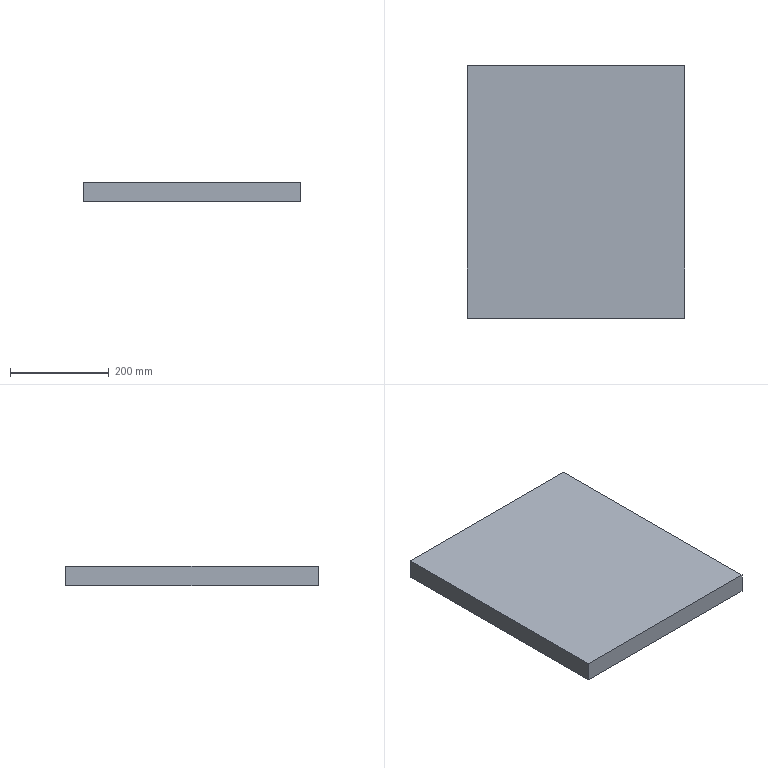Part | SolidWorks | features Extrusion 1 | 1 solid | 6 faces | box 440 x 510 x 40 mm | volume 8976000 mm3 | plane 6
STEP:
#1=CARTESIAN_POINT('',(0.,510.,0.));
#2=VERTEX_POINT('',#1);
#3=CARTESIAN_POINT('',(0.,0.,0.));
#4=VERTEX_POINT('',#3);
#5=CARTESIAN_POINT('',(0.,0.,0.));
#6=DIRECTION('',(0.,-1.,0.));
#7=VECTOR('',#6,1000.);
#8=LINE('',#5,#7);
#9=EDGE_CURVE('',#2,#4,#8,.T.);
#10=ORIENTED_EDGE('',*,*,#9,.T.);
#11=CARTESIAN_POINT('',(0.,0.,40.));
#12=VERTEX_POINT('',#11);
#13=CARTESIAN_POINT('',(0.,0.,40.));
#14=DIRECTION('',(0.,0.,-1.));
#15=VECTOR('',#14,1000.);
#16=LINE('',#13,#15);
#17=EDGE_CURVE('',#12,#4,#16,.T.);
#18=ORIENTED_EDGE('',*,*,#17,.F.);
#19=CARTESIAN_POINT('',(0.,510.,40.));
#20=VERTEX_POINT('',#19);
#21=CARTESIAN_POINT('',(0.,0.,40.));
#22=DIRECTION('',(0.,-1.,0.));
#23=VECTOR('',#22,1000.);
#24=LINE('',#21,#23);
#25=EDGE_CURVE('',#20,#12,#24,.T.);
#26=ORIENTED_EDGE('',*,*,#25,.F.);
#27=CARTESIAN_POINT('',(0.,510.,40.));
#28=DIRECTION('',(0.,0.,-1.));
#29=VECTOR('',#28,1000.);
#30=LINE('',#27,#29);
#31=EDGE_CURVE('',#20,#2,#30,.T.);
#32=ORIENTED_EDGE('',*,*,#31,.T.);
#33=EDGE_LOOP('',(#10,#18,#26,#32));
#34=FACE_OUTER_BOUND('',#33,.T.);
#35=CARTESIAN_POINT('',(0.,0.,40.));
#36=DIRECTION('',(1.,0.,0.));
#37=DIRECTION('',(0.,0.,-1.));
#38=AXIS2_PLACEMENT_3D('',#35,#36,#37);
#39=PLANE('',#38);
#40=ADVANCED_FACE('',(#34),#39,.F.);
#41=CARTESIAN_POINT('',(440.,0.,0.));
#42=VERTEX_POINT('',#41);
#43=CARTESIAN_POINT('',(0.,0.,0.));
#44=DIRECTION('',(1.,0.,0.));
#45=VECTOR('',#44,1000.);
#46=LINE('',#43,#45);
#47=EDGE_CURVE('',#4,#42,#46,.T.);
#48=ORIENTED_EDGE('',*,*,#47,.T.);
#49=CARTESIAN_POINT('',(440.,0.,40.));
#50=VERTEX_POINT('',#49);
#51=CARTESIAN_POINT('',(440.,0.,40.));
#52=DIRECTION('',(0.,0.,-1.));
#53=VECTOR('',#52,1000.);
#54=LINE('',#51,#53);
#55=EDGE_CURVE('',#50,#42,#54,.T.);
#56=ORIENTED_EDGE('',*,*,#55,.F.);
#57=CARTESIAN_POINT('',(0.,0.,40.));
#58=DIRECTION('',(1.,0.,0.));
#59=VECTOR('',#58,1000.);
#60=LINE('',#57,#59);
#61=EDGE_CURVE('',#12,#50,#60,.T.);
#62=ORIENTED_EDGE('',*,*,#61,.F.);
#63=ORIENTED_EDGE('',*,*,#17,.T.);
#64=EDGE_LOOP('',(#48,#56,#62,#63));
#65=FACE_OUTER_BOUND('',#64,.T.);
#66=CARTESIAN_POINT('',(0.,0.,40.));
#67=DIRECTION('',(0.,1.,0.));
#68=DIRECTION('',(0.,0.,1.));
#69=AXIS2_PLACEMENT_3D('',#66,#67,#68);
#70=PLANE('',#69);
#71=ADVANCED_FACE('',(#65),#70,.F.);
#72=CARTESIAN_POINT('',(440.,510.,0.));
#73=VERTEX_POINT('',#72);
#74=CARTESIAN_POINT('',(440.,0.,0.));
#75=DIRECTION('',(0.,1.,0.));
#76=VECTOR('',#75,1000.);
#77=LINE('',#74,#76);
#78=EDGE_CURVE('',#42,#73,#77,.T.);
#79=ORIENTED_EDGE('',*,*,#78,.T.);
#80=CARTESIAN_POINT('',(440.,510.,40.));
#81=VERTEX_POINT('',#80);
#82=CARTESIAN_POINT('',(440.,510.,40.));
#83=DIRECTION('',(0.,0.,-1.));
#84=VECTOR('',#83,1000.);
#85=LINE('',#82,#84);
#86=EDGE_CURVE('',#81,#73,#85,.T.);
#87=ORIENTED_EDGE('',*,*,#86,.F.);
#88=CARTESIAN_POINT('',(440.,0.,40.));
#89=DIRECTION('',(0.,1.,0.));
#90=VECTOR('',#89,1000.);
#91=LINE('',#88,#90);
#92=EDGE_CURVE('',#50,#81,#91,.T.);
#93=ORIENTED_EDGE('',*,*,#92,.F.);
#94=ORIENTED_EDGE('',*,*,#55,.T.);
#95=EDGE_LOOP('',(#79,#87,#93,#94));
#96=FACE_OUTER_BOUND('',#95,.T.);
#97=CARTESIAN_POINT('',(440.,0.,40.));
#98=DIRECTION('',(-1.,0.,0.));
#99=DIRECTION('',(0.,0.,1.));
#100=AXIS2_PLACEMENT_3D('',#97,#98,#99);
#101=PLANE('',#100);
#102=ADVANCED_FACE('',(#96),#101,.F.);
#103=CARTESIAN_POINT('',(0.,510.,0.));
#104=DIRECTION('',(-1.,0.,0.));
#105=VECTOR('',#104,1000.);
#106=LINE('',#103,#105);
#107=EDGE_CURVE('',#73,#2,#106,.T.);
#108=ORIENTED_EDGE('',*,*,#107,.T.);
#109=ORIENTED_EDGE('',*,*,#31,.F.);
#110=CARTESIAN_POINT('',(0.,510.,40.));
#111=DIRECTION('',(-1.,0.,0.));
#112=VECTOR('',#111,1000.);
#113=LINE('',#110,#112);
#114=EDGE_CURVE('',#81,#20,#113,.T.);
#115=ORIENTED_EDGE('',*,*,#114,.F.);
#116=ORIENTED_EDGE('',*,*,#86,.T.);
#117=EDGE_LOOP('',(#108,#109,#115,#116));
#118=FACE_OUTER_BOUND('',#117,.T.);
#119=CARTESIAN_POINT('',(0.,510.,40.));
#120=DIRECTION('',(0.,-1.,0.));
#121=DIRECTION('',(0.,0.,-1.));
#122=AXIS2_PLACEMENT_3D('',#119,#120,#121);
#123=PLANE('',#122);
#124=ADVANCED_FACE('',(#118),#123,.F.);
#125=ORIENTED_EDGE('',*,*,#25,.T.);
#126=ORIENTED_EDGE('',*,*,#61,.T.);
#127=ORIENTED_EDGE('',*,*,#92,.T.);
#128=ORIENTED_EDGE('',*,*,#114,.T.);
#129=EDGE_LOOP('',(#125,#126,#127,#128));
#130=FACE_OUTER_BOUND('',#129,.T.);
#131=CARTESIAN_POINT('',(0.,0.,40.));
#132=DIRECTION('',(0.,0.,-1.));
#133=DIRECTION('',(-1.,0.,0.));
#134=AXIS2_PLACEMENT_3D('',#131,#132,#133);
#135=PLANE('',#134);
#136=ADVANCED_FACE('',(#130),#135,.F.);
#137=ORIENTED_EDGE('',*,*,#9,.F.);
#138=ORIENTED_EDGE('',*,*,#107,.F.);
#139=ORIENTED_EDGE('',*,*,#78,.F.);
#140=ORIENTED_EDGE('',*,*,#47,.F.);
#141=EDGE_LOOP('',(#137,#138,#139,#140));
#142=FACE_OUTER_BOUND('',#141,.T.);
#143=CARTESIAN_POINT('',(0.,0.,0.));
#144=DIRECTION('',(0.,0.,-1.));
#145=DIRECTION('',(-1.,0.,0.));
#146=AXIS2_PLACEMENT_3D('',#143,#144,#145);
#147=PLANE('',#146);
#148=ADVANCED_FACE('',(#142),#147,.T.);
#149=CLOSED_SHELL('',(#40,#71,#102,#124,#136,#148));
#150=MANIFOLD_SOLID_BREP('',#149);
#151=CARTESIAN_POINT('',(0.,0.,0.));
#152=DIRECTION('',(0.,0.,1.));
#153=DIRECTION('',(1.,0.,0.));
#154=AXIS2_PLACEMENT_3D('',#151,#152,#153);
#155=(LENGTH_UNIT()NAMED_UNIT(*)SI_UNIT(.MILLI.,.METRE.));
#156=UNCERTAINTY_MEASURE_WITH_UNIT(LENGTH_MEASURE(0.00001),#155,'','');
#157=(NAMED_UNIT(*)PLANE_ANGLE_UNIT()SI_UNIT($,.RADIAN.));
#158=(NAMED_UNIT(*)SI_UNIT($,.STERADIAN.)SOLID_ANGLE_UNIT());
#159=(GEOMETRIC_REPRESENTATION_CONTEXT(3)GLOBAL_UNCERTAINTY_ASSIGNED_CONTEXT((#156))GLOBAL_UNIT_ASSIGNED_CONTEXT((#155,#157,#158))REPRESENTATION_CONTEXT('',''));
#160=ADVANCED_BREP_SHAPE_REPRESENTATION('',(#150,#154),#159);